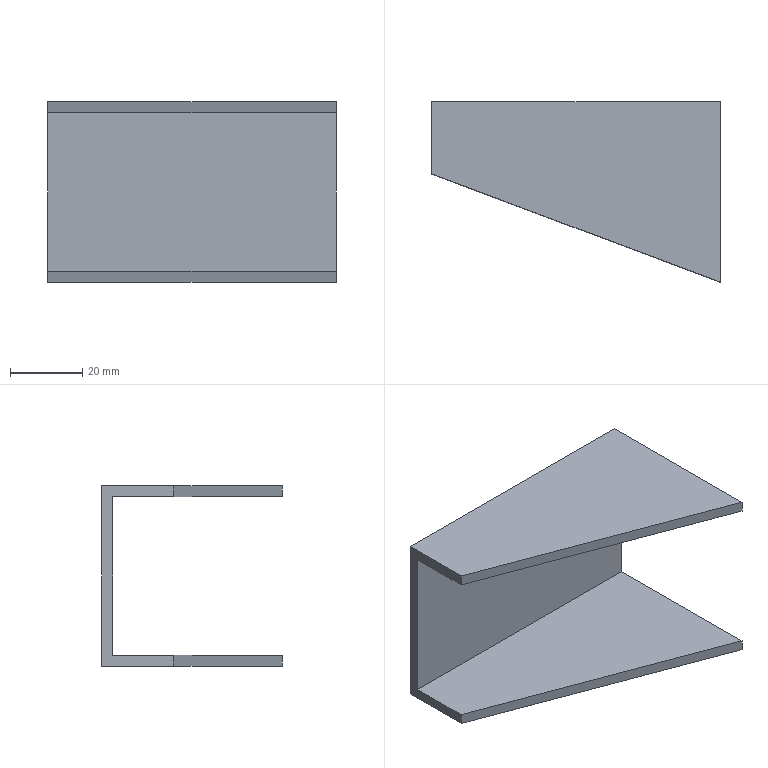Part | SolidWorks | features Extrusion 1, Shell 1 | 1 solid | 10 faces | box 80 x 50 x 50 mm | volume 27360 mm3 | plane 10
STEP:
#1=CARTESIAN_POINT('',(-80.,30.,3.));
#2=VERTEX_POINT('',#1);
#3=CARTESIAN_POINT('',(0.,0.,3.));
#4=VERTEX_POINT('',#3);
#5=CARTESIAN_POINT('',(-80.,30.,3.));
#6=DIRECTION('',(0.9363,-0.3511,0.));
#7=VECTOR('',#6,1000.);
#8=LINE('',#5,#7);
#9=EDGE_CURVE('',#2,#4,#8,.T.);
#10=ORIENTED_EDGE('',*,*,#9,.F.);
#11=CARTESIAN_POINT('',(-80.,30.,0.));
#12=VERTEX_POINT('',#11);
#13=CARTESIAN_POINT('',(-80.,30.,50.));
#14=DIRECTION('',(0.,0.,-1.));
#15=VECTOR('',#14,1000.);
#16=LINE('',#13,#15);
#17=EDGE_CURVE('',#2,#12,#16,.T.);
#18=ORIENTED_EDGE('',*,*,#17,.T.);
#19=CARTESIAN_POINT('',(0.,0.,0.));
#20=VERTEX_POINT('',#19);
#21=CARTESIAN_POINT('',(-80.,30.,0.));
#22=DIRECTION('',(0.9363,-0.3511,0.));
#23=VECTOR('',#22,1000.);
#24=LINE('',#21,#23);
#25=EDGE_CURVE('',#12,#20,#24,.T.);
#26=ORIENTED_EDGE('',*,*,#25,.T.);
#27=CARTESIAN_POINT('',(0.,0.,50.));
#28=DIRECTION('',(0.,0.,-1.));
#29=VECTOR('',#28,1000.);
#30=LINE('',#27,#29);
#31=EDGE_CURVE('',#4,#20,#30,.T.);
#32=ORIENTED_EDGE('',*,*,#31,.F.);
#33=EDGE_LOOP('',(#10,#18,#26,#32));
#34=FACE_OUTER_BOUND('',#33,.T.);
#35=CARTESIAN_POINT('',(-80.,30.,50.));
#36=DIRECTION('',(0.3511,0.9363,0.));
#37=DIRECTION('',(-0.9363,0.3511,0.));
#38=AXIS2_PLACEMENT_3D('',#35,#36,#37);
#39=PLANE('',#38);
#40=ADVANCED_FACE('',(#34),#39,.F.);
#41=CARTESIAN_POINT('',(0.,47.,3.));
#42=VERTEX_POINT('',#41);
#43=CARTESIAN_POINT('',(0.,0.,3.));
#44=DIRECTION('',(0.,1.,0.));
#45=VECTOR('',#44,1000.);
#46=LINE('',#43,#45);
#47=EDGE_CURVE('',#4,#42,#46,.T.);
#48=ORIENTED_EDGE('',*,*,#47,.F.);
#49=ORIENTED_EDGE('',*,*,#31,.T.);
#50=CARTESIAN_POINT('',(0.,50.,0.));
#51=VERTEX_POINT('',#50);
#52=CARTESIAN_POINT('',(0.,0.,0.));
#53=DIRECTION('',(0.,1.,0.));
#54=VECTOR('',#53,1000.);
#55=LINE('',#52,#54);
#56=EDGE_CURVE('',#20,#51,#55,.T.);
#57=ORIENTED_EDGE('',*,*,#56,.T.);
#58=CARTESIAN_POINT('',(0.,50.,50.));
#59=VERTEX_POINT('',#58);
#60=CARTESIAN_POINT('',(0.,50.,50.));
#61=DIRECTION('',(0.,0.,-1.));
#62=VECTOR('',#61,1000.);
#63=LINE('',#60,#62);
#64=EDGE_CURVE('',#59,#51,#63,.T.);
#65=ORIENTED_EDGE('',*,*,#64,.F.);
#66=CARTESIAN_POINT('',(0.,0.,50.));
#67=VERTEX_POINT('',#66);
#68=CARTESIAN_POINT('',(0.,0.,50.));
#69=DIRECTION('',(0.,1.,0.));
#70=VECTOR('',#69,1000.);
#71=LINE('',#68,#70);
#72=EDGE_CURVE('',#67,#59,#71,.T.);
#73=ORIENTED_EDGE('',*,*,#72,.F.);
#74=CARTESIAN_POINT('',(0.,0.,47.));
#75=VERTEX_POINT('',#74);
#76=CARTESIAN_POINT('',(0.,0.,50.));
#77=DIRECTION('',(0.,0.,-1.));
#78=VECTOR('',#77,1000.);
#79=LINE('',#76,#78);
#80=EDGE_CURVE('',#67,#75,#79,.T.);
#81=ORIENTED_EDGE('',*,*,#80,.T.);
#82=CARTESIAN_POINT('',(0.,47.,47.));
#83=VERTEX_POINT('',#82);
#84=CARTESIAN_POINT('',(0.,0.,47.));
#85=DIRECTION('',(0.,1.,0.));
#86=VECTOR('',#85,1000.);
#87=LINE('',#84,#86);
#88=EDGE_CURVE('',#75,#83,#87,.T.);
#89=ORIENTED_EDGE('',*,*,#88,.T.);
#90=CARTESIAN_POINT('',(0.,47.,50.));
#91=DIRECTION('',(0.,0.,-1.));
#92=VECTOR('',#91,1000.);
#93=LINE('',#90,#92);
#94=EDGE_CURVE('',#83,#42,#93,.T.);
#95=ORIENTED_EDGE('',*,*,#94,.T.);
#96=EDGE_LOOP('',(#48,#49,#57,#65,#73,#81,#89,#95));
#97=FACE_OUTER_BOUND('',#96,.T.);
#98=CARTESIAN_POINT('',(0.,0.,50.));
#99=DIRECTION('',(-1.,0.,0.));
#100=DIRECTION('',(0.,0.,1.));
#101=AXIS2_PLACEMENT_3D('',#98,#99,#100);
#102=PLANE('',#101);
#103=ADVANCED_FACE('',(#97),#102,.F.);
#104=CARTESIAN_POINT('',(-80.,47.,3.));
#105=VERTEX_POINT('',#104);
#106=CARTESIAN_POINT('',(-80.,50.,3.));
#107=DIRECTION('',(0.,-1.,0.));
#108=VECTOR('',#107,1000.);
#109=LINE('',#106,#108);
#110=EDGE_CURVE('',#105,#2,#109,.T.);
#111=ORIENTED_EDGE('',*,*,#110,.F.);
#112=CARTESIAN_POINT('',(-80.,47.,47.));
#113=VERTEX_POINT('',#112);
#114=CARTESIAN_POINT('',(-80.,47.,50.));
#115=DIRECTION('',(0.,0.,-1.));
#116=VECTOR('',#115,1000.);
#117=LINE('',#114,#116);
#118=EDGE_CURVE('',#113,#105,#117,.T.);
#119=ORIENTED_EDGE('',*,*,#118,.F.);
#120=CARTESIAN_POINT('',(-80.,30.,47.));
#121=VERTEX_POINT('',#120);
#122=CARTESIAN_POINT('',(-80.,50.,47.));
#123=DIRECTION('',(0.,-1.,0.));
#124=VECTOR('',#123,1000.);
#125=LINE('',#122,#124);
#126=EDGE_CURVE('',#113,#121,#125,.T.);
#127=ORIENTED_EDGE('',*,*,#126,.T.);
#128=CARTESIAN_POINT('',(-80.,30.,50.));
#129=VERTEX_POINT('',#128);
#130=CARTESIAN_POINT('',(-80.,30.,50.));
#131=DIRECTION('',(0.,0.,-1.));
#132=VECTOR('',#131,1000.);
#133=LINE('',#130,#132);
#134=EDGE_CURVE('',#129,#121,#133,.T.);
#135=ORIENTED_EDGE('',*,*,#134,.F.);
#136=CARTESIAN_POINT('',(-80.,50.,50.));
#137=VERTEX_POINT('',#136);
#138=CARTESIAN_POINT('',(-80.,50.,50.));
#139=DIRECTION('',(0.,-1.,0.));
#140=VECTOR('',#139,1000.);
#141=LINE('',#138,#140);
#142=EDGE_CURVE('',#137,#129,#141,.T.);
#143=ORIENTED_EDGE('',*,*,#142,.F.);
#144=CARTESIAN_POINT('',(-80.,50.,0.));
#145=VERTEX_POINT('',#144);
#146=CARTESIAN_POINT('',(-80.,50.,50.));
#147=DIRECTION('',(0.,0.,-1.));
#148=VECTOR('',#147,1000.);
#149=LINE('',#146,#148);
#150=EDGE_CURVE('',#137,#145,#149,.T.);
#151=ORIENTED_EDGE('',*,*,#150,.T.);
#152=CARTESIAN_POINT('',(-80.,50.,0.));
#153=DIRECTION('',(0.,-1.,0.));
#154=VECTOR('',#153,1000.);
#155=LINE('',#152,#154);
#156=EDGE_CURVE('',#145,#12,#155,.T.);
#157=ORIENTED_EDGE('',*,*,#156,.T.);
#158=ORIENTED_EDGE('',*,*,#17,.F.);
#159=EDGE_LOOP('',(#111,#119,#127,#135,#143,#151,#157,#158));
#160=FACE_OUTER_BOUND('',#159,.T.);
#161=CARTESIAN_POINT('',(-80.,50.,50.));
#162=DIRECTION('',(1.,0.,0.));
#163=DIRECTION('',(0.,0.,-1.));
#164=AXIS2_PLACEMENT_3D('',#161,#162,#163);
#165=PLANE('',#164);
#166=ADVANCED_FACE('',(#160),#165,.F.);
#167=ORIENTED_EDGE('',*,*,#134,.T.);
#168=CARTESIAN_POINT('',(-80.,30.,47.));
#169=DIRECTION('',(0.9363,-0.3511,0.));
#170=VECTOR('',#169,1000.);
#171=LINE('',#168,#170);
#172=EDGE_CURVE('',#121,#75,#171,.T.);
#173=ORIENTED_EDGE('',*,*,#172,.T.);
#174=ORIENTED_EDGE('',*,*,#80,.F.);
#175=CARTESIAN_POINT('',(-80.,30.,50.));
#176=DIRECTION('',(0.9363,-0.3511,0.));
#177=VECTOR('',#176,1000.);
#178=LINE('',#175,#177);
#179=EDGE_CURVE('',#129,#67,#178,.T.);
#180=ORIENTED_EDGE('',*,*,#179,.F.);
#181=EDGE_LOOP('',(#167,#173,#174,#180));
#182=FACE_OUTER_BOUND('',#181,.T.);
#183=CARTESIAN_POINT('',(-80.,30.,50.));
#184=DIRECTION('',(0.3511,0.9363,0.));
#185=DIRECTION('',(-0.9363,0.3511,0.));
#186=AXIS2_PLACEMENT_3D('',#183,#184,#185);
#187=PLANE('',#186);
#188=ADVANCED_FACE('',(#182),#187,.F.);
#189=CARTESIAN_POINT('',(0.,50.,0.));
#190=DIRECTION('',(-1.,0.,0.));
#191=VECTOR('',#190,1000.);
#192=LINE('',#189,#191);
#193=EDGE_CURVE('',#51,#145,#192,.T.);
#194=ORIENTED_EDGE('',*,*,#193,.T.);
#195=ORIENTED_EDGE('',*,*,#150,.F.);
#196=CARTESIAN_POINT('',(0.,50.,50.));
#197=DIRECTION('',(-1.,0.,0.));
#198=VECTOR('',#197,1000.);
#199=LINE('',#196,#198);
#200=EDGE_CURVE('',#59,#137,#199,.T.);
#201=ORIENTED_EDGE('',*,*,#200,.F.);
#202=ORIENTED_EDGE('',*,*,#64,.T.);
#203=EDGE_LOOP('',(#194,#195,#201,#202));
#204=FACE_OUTER_BOUND('',#203,.T.);
#205=CARTESIAN_POINT('',(0.,50.,50.));
#206=DIRECTION('',(0.,-1.,0.));
#207=DIRECTION('',(1.,0.,0.));
#208=AXIS2_PLACEMENT_3D('',#205,#206,#207);
#209=PLANE('',#208);
#210=ADVANCED_FACE('',(#204),#209,.F.);
#211=ORIENTED_EDGE('',*,*,#179,.T.);
#212=ORIENTED_EDGE('',*,*,#72,.T.);
#213=ORIENTED_EDGE('',*,*,#200,.T.);
#214=ORIENTED_EDGE('',*,*,#142,.T.);
#215=EDGE_LOOP('',(#211,#212,#213,#214));
#216=FACE_OUTER_BOUND('',#215,.T.);
#217=CARTESIAN_POINT('',(0.,0.,50.));
#218=DIRECTION('',(0.,0.,1.));
#219=DIRECTION('',(1.,0.,0.));
#220=AXIS2_PLACEMENT_3D('',#217,#218,#219);
#221=PLANE('',#220);
#222=ADVANCED_FACE('',(#216),#221,.T.);
#223=ORIENTED_EDGE('',*,*,#25,.F.);
#224=ORIENTED_EDGE('',*,*,#156,.F.);
#225=ORIENTED_EDGE('',*,*,#193,.F.);
#226=ORIENTED_EDGE('',*,*,#56,.F.);
#227=EDGE_LOOP('',(#223,#224,#225,#226));
#228=FACE_OUTER_BOUND('',#227,.T.);
#229=CARTESIAN_POINT('',(0.,0.,0.));
#230=DIRECTION('',(0.,0.,1.));
#231=DIRECTION('',(1.,0.,0.));
#232=AXIS2_PLACEMENT_3D('',#229,#230,#231);
#233=PLANE('',#232);
#234=ADVANCED_FACE('',(#228),#233,.F.);
#235=CARTESIAN_POINT('',(0.,47.,3.));
#236=DIRECTION('',(-1.,0.,0.));
#237=VECTOR('',#236,1000.);
#238=LINE('',#235,#237);
#239=EDGE_CURVE('',#42,#105,#238,.T.);
#240=ORIENTED_EDGE('',*,*,#239,.F.);
#241=ORIENTED_EDGE('',*,*,#94,.F.);
#242=CARTESIAN_POINT('',(0.,47.,47.));
#243=DIRECTION('',(-1.,0.,0.));
#244=VECTOR('',#243,1000.);
#245=LINE('',#242,#244);
#246=EDGE_CURVE('',#83,#113,#245,.T.);
#247=ORIENTED_EDGE('',*,*,#246,.T.);
#248=ORIENTED_EDGE('',*,*,#118,.T.);
#249=EDGE_LOOP('',(#240,#241,#247,#248));
#250=FACE_OUTER_BOUND('',#249,.T.);
#251=CARTESIAN_POINT('',(0.,47.,50.));
#252=DIRECTION('',(0.,-1.,0.));
#253=DIRECTION('',(1.,0.,0.));
#254=AXIS2_PLACEMENT_3D('',#251,#252,#253);
#255=PLANE('',#254);
#256=ADVANCED_FACE('',(#250),#255,.T.);
#257=ORIENTED_EDGE('',*,*,#172,.F.);
#258=ORIENTED_EDGE('',*,*,#126,.F.);
#259=ORIENTED_EDGE('',*,*,#246,.F.);
#260=ORIENTED_EDGE('',*,*,#88,.F.);
#261=EDGE_LOOP('',(#257,#258,#259,#260));
#262=FACE_OUTER_BOUND('',#261,.T.);
#263=CARTESIAN_POINT('',(0.,0.,47.));
#264=DIRECTION('',(0.,0.,1.));
#265=DIRECTION('',(1.,0.,0.));
#266=AXIS2_PLACEMENT_3D('',#263,#264,#265);
#267=PLANE('',#266);
#268=ADVANCED_FACE('',(#262),#267,.F.);
#269=ORIENTED_EDGE('',*,*,#9,.T.);
#270=ORIENTED_EDGE('',*,*,#47,.T.);
#271=ORIENTED_EDGE('',*,*,#239,.T.);
#272=ORIENTED_EDGE('',*,*,#110,.T.);
#273=EDGE_LOOP('',(#269,#270,#271,#272));
#274=FACE_OUTER_BOUND('',#273,.T.);
#275=CARTESIAN_POINT('',(0.,0.,3.));
#276=DIRECTION('',(0.,0.,1.));
#277=DIRECTION('',(1.,0.,0.));
#278=AXIS2_PLACEMENT_3D('',#275,#276,#277);
#279=PLANE('',#278);
#280=ADVANCED_FACE('',(#274),#279,.T.);
#281=CLOSED_SHELL('',(#40,#103,#166,#188,#210,#222,#234,#256,#268,#280));
#282=MANIFOLD_SOLID_BREP('',#281);
#283=CARTESIAN_POINT('',(0.,0.,0.));
#284=DIRECTION('',(0.,0.,1.));
#285=DIRECTION('',(1.,0.,0.));
#286=AXIS2_PLACEMENT_3D('',#283,#284,#285);
#287=(LENGTH_UNIT()NAMED_UNIT(*)SI_UNIT(.MILLI.,.METRE.));
#288=UNCERTAINTY_MEASURE_WITH_UNIT(LENGTH_MEASURE(0.00001),#287,'','');
#289=(NAMED_UNIT(*)PLANE_ANGLE_UNIT()SI_UNIT($,.RADIAN.));
#290=(NAMED_UNIT(*)SI_UNIT($,.STERADIAN.)SOLID_ANGLE_UNIT());
#291=(GEOMETRIC_REPRESENTATION_CONTEXT(3)GLOBAL_UNCERTAINTY_ASSIGNED_CONTEXT((#288))GLOBAL_UNIT_ASSIGNED_CONTEXT((#287,#289,#290))REPRESENTATION_CONTEXT('',''));
#292=ADVANCED_BREP_SHAPE_REPRESENTATION('',(#282,#286),#291);